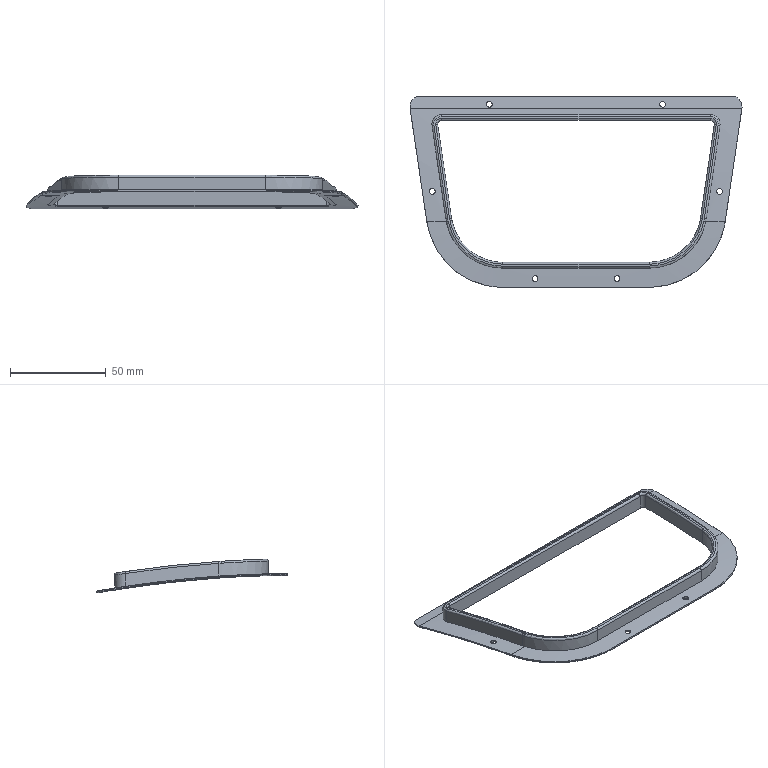Part | SolidWorks | features SplitBody 1 | 1 solid | 90 faces | box 173.097 x 99.379 x 17.536 mm | volume 14952 mm3 | spline 39 | cylinder 36 | plane 15 | commonest cylinder face diameters 3 x12 10 x6 2 x4 4 x3 12 x3 1 x2